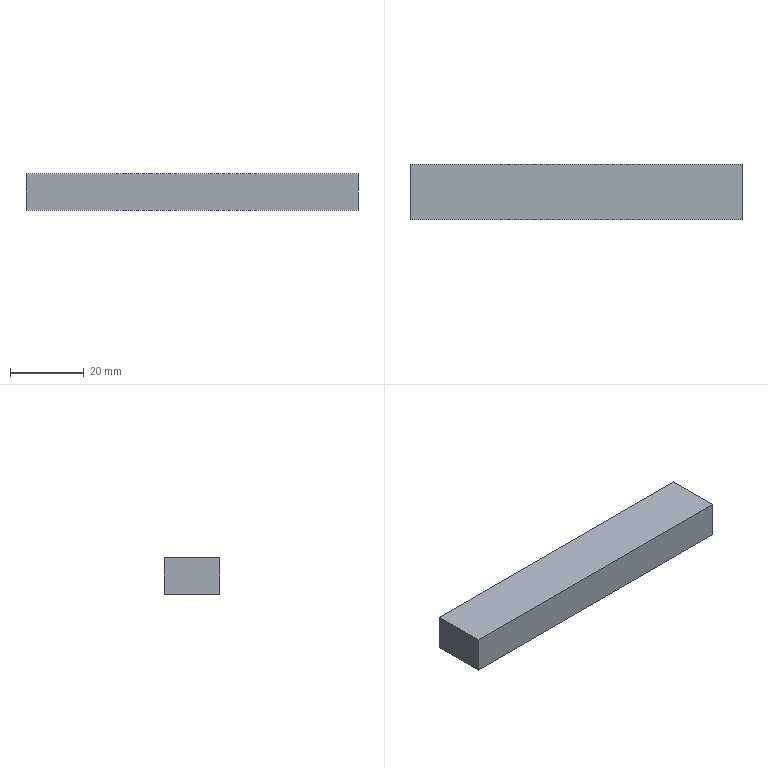Part | SolidWorks | features BaseBody 1 | 1 solid | 6 faces | box 90 x 15 x 10 mm | volume 13500 mm3 | plane 6
STEP:
#1=CARTESIAN_POINT('',(45.,-7.5,0.));
#2=VERTEX_POINT('',#1);
#3=CARTESIAN_POINT('',(45.,7.5,0.));
#4=VERTEX_POINT('',#3);
#5=CARTESIAN_POINT('',(45.,7.5,0.));
#6=DIRECTION('',(0.,1.,0.));
#7=VECTOR('',#6,1000.);
#8=LINE('',#5,#7);
#9=EDGE_CURVE('',#2,#4,#8,.T.);
#10=ORIENTED_EDGE('',*,*,#9,.T.);
#11=CARTESIAN_POINT('',(45.,7.5,10.));
#12=VERTEX_POINT('',#11);
#13=CARTESIAN_POINT('',(45.,7.5,10.));
#14=DIRECTION('',(0.,0.,-1.));
#15=VECTOR('',#14,1000.);
#16=LINE('',#13,#15);
#17=EDGE_CURVE('',#12,#4,#16,.T.);
#18=ORIENTED_EDGE('',*,*,#17,.F.);
#19=CARTESIAN_POINT('',(45.,-7.5,10.));
#20=VERTEX_POINT('',#19);
#21=CARTESIAN_POINT('',(45.,7.5,10.));
#22=DIRECTION('',(0.,1.,0.));
#23=VECTOR('',#22,1000.);
#24=LINE('',#21,#23);
#25=EDGE_CURVE('',#20,#12,#24,.T.);
#26=ORIENTED_EDGE('',*,*,#25,.F.);
#27=CARTESIAN_POINT('',(45.,-7.5,10.));
#28=DIRECTION('',(0.,0.,-1.));
#29=VECTOR('',#28,1000.);
#30=LINE('',#27,#29);
#31=EDGE_CURVE('',#20,#2,#30,.T.);
#32=ORIENTED_EDGE('',*,*,#31,.T.);
#33=EDGE_LOOP('',(#10,#18,#26,#32));
#34=FACE_OUTER_BOUND('',#33,.T.);
#35=CARTESIAN_POINT('',(45.,7.5,10.));
#36=DIRECTION('',(-1.,0.,0.));
#37=DIRECTION('',(0.,0.,1.));
#38=AXIS2_PLACEMENT_3D('',#35,#36,#37);
#39=PLANE('',#38);
#40=ADVANCED_FACE('',(#34),#39,.F.);
#41=CARTESIAN_POINT('',(-45.,7.5,0.));
#42=VERTEX_POINT('',#41);
#43=CARTESIAN_POINT('',(-45.,7.5,0.));
#44=DIRECTION('',(-1.,0.,0.));
#45=VECTOR('',#44,1000.);
#46=LINE('',#43,#45);
#47=EDGE_CURVE('',#4,#42,#46,.T.);
#48=ORIENTED_EDGE('',*,*,#47,.T.);
#49=CARTESIAN_POINT('',(-45.,7.5,10.));
#50=VERTEX_POINT('',#49);
#51=CARTESIAN_POINT('',(-45.,7.5,10.));
#52=DIRECTION('',(0.,0.,-1.));
#53=VECTOR('',#52,1000.);
#54=LINE('',#51,#53);
#55=EDGE_CURVE('',#50,#42,#54,.T.);
#56=ORIENTED_EDGE('',*,*,#55,.F.);
#57=CARTESIAN_POINT('',(-45.,7.5,10.));
#58=DIRECTION('',(-1.,0.,0.));
#59=VECTOR('',#58,1000.);
#60=LINE('',#57,#59);
#61=EDGE_CURVE('',#12,#50,#60,.T.);
#62=ORIENTED_EDGE('',*,*,#61,.F.);
#63=ORIENTED_EDGE('',*,*,#17,.T.);
#64=EDGE_LOOP('',(#48,#56,#62,#63));
#65=FACE_OUTER_BOUND('',#64,.T.);
#66=CARTESIAN_POINT('',(-45.,7.5,10.));
#67=DIRECTION('',(0.,-1.,0.));
#68=DIRECTION('',(0.,0.,-1.));
#69=AXIS2_PLACEMENT_3D('',#66,#67,#68);
#70=PLANE('',#69);
#71=ADVANCED_FACE('',(#65),#70,.F.);
#72=CARTESIAN_POINT('',(-45.,-7.5,0.));
#73=VERTEX_POINT('',#72);
#74=CARTESIAN_POINT('',(-45.,7.5,0.));
#75=DIRECTION('',(0.,-1.,0.));
#76=VECTOR('',#75,1000.);
#77=LINE('',#74,#76);
#78=EDGE_CURVE('',#42,#73,#77,.T.);
#79=ORIENTED_EDGE('',*,*,#78,.T.);
#80=CARTESIAN_POINT('',(-45.,-7.5,10.));
#81=VERTEX_POINT('',#80);
#82=CARTESIAN_POINT('',(-45.,-7.5,10.));
#83=DIRECTION('',(0.,0.,-1.));
#84=VECTOR('',#83,1000.);
#85=LINE('',#82,#84);
#86=EDGE_CURVE('',#81,#73,#85,.T.);
#87=ORIENTED_EDGE('',*,*,#86,.F.);
#88=CARTESIAN_POINT('',(-45.,7.5,10.));
#89=DIRECTION('',(0.,-1.,0.));
#90=VECTOR('',#89,1000.);
#91=LINE('',#88,#90);
#92=EDGE_CURVE('',#50,#81,#91,.T.);
#93=ORIENTED_EDGE('',*,*,#92,.F.);
#94=ORIENTED_EDGE('',*,*,#55,.T.);
#95=EDGE_LOOP('',(#79,#87,#93,#94));
#96=FACE_OUTER_BOUND('',#95,.T.);
#97=CARTESIAN_POINT('',(-45.,7.5,10.));
#98=DIRECTION('',(1.,0.,0.));
#99=DIRECTION('',(0.,0.,-1.));
#100=AXIS2_PLACEMENT_3D('',#97,#98,#99);
#101=PLANE('',#100);
#102=ADVANCED_FACE('',(#96),#101,.F.);
#103=CARTESIAN_POINT('',(-45.,-7.5,0.));
#104=DIRECTION('',(1.,0.,0.));
#105=VECTOR('',#104,1000.);
#106=LINE('',#103,#105);
#107=EDGE_CURVE('',#73,#2,#106,.T.);
#108=ORIENTED_EDGE('',*,*,#107,.T.);
#109=ORIENTED_EDGE('',*,*,#31,.F.);
#110=CARTESIAN_POINT('',(-45.,-7.5,10.));
#111=DIRECTION('',(1.,0.,0.));
#112=VECTOR('',#111,1000.);
#113=LINE('',#110,#112);
#114=EDGE_CURVE('',#81,#20,#113,.T.);
#115=ORIENTED_EDGE('',*,*,#114,.F.);
#116=ORIENTED_EDGE('',*,*,#86,.T.);
#117=EDGE_LOOP('',(#108,#109,#115,#116));
#118=FACE_OUTER_BOUND('',#117,.T.);
#119=CARTESIAN_POINT('',(-45.,-7.5,10.));
#120=DIRECTION('',(0.,1.,0.));
#121=DIRECTION('',(0.,0.,1.));
#122=AXIS2_PLACEMENT_3D('',#119,#120,#121);
#123=PLANE('',#122);
#124=ADVANCED_FACE('',(#118),#123,.F.);
#125=ORIENTED_EDGE('',*,*,#25,.T.);
#126=ORIENTED_EDGE('',*,*,#61,.T.);
#127=ORIENTED_EDGE('',*,*,#92,.T.);
#128=ORIENTED_EDGE('',*,*,#114,.T.);
#129=EDGE_LOOP('',(#125,#126,#127,#128));
#130=FACE_OUTER_BOUND('',#129,.T.);
#131=CARTESIAN_POINT('',(0.,0.,10.));
#132=DIRECTION('',(0.,0.,1.));
#133=DIRECTION('',(1.,0.,0.));
#134=AXIS2_PLACEMENT_3D('',#131,#132,#133);
#135=PLANE('',#134);
#136=ADVANCED_FACE('',(#130),#135,.T.);
#137=ORIENTED_EDGE('',*,*,#9,.F.);
#138=ORIENTED_EDGE('',*,*,#107,.F.);
#139=ORIENTED_EDGE('',*,*,#78,.F.);
#140=ORIENTED_EDGE('',*,*,#47,.F.);
#141=EDGE_LOOP('',(#137,#138,#139,#140));
#142=FACE_OUTER_BOUND('',#141,.T.);
#143=CARTESIAN_POINT('',(0.,0.,0.));
#144=DIRECTION('',(0.,0.,1.));
#145=DIRECTION('',(1.,0.,0.));
#146=AXIS2_PLACEMENT_3D('',#143,#144,#145);
#147=PLANE('',#146);
#148=ADVANCED_FACE('',(#142),#147,.F.);
#149=CLOSED_SHELL('',(#40,#71,#102,#124,#136,#148));
#150=MANIFOLD_SOLID_BREP('',#149);
#151=CARTESIAN_POINT('',(0.,0.,0.));
#152=DIRECTION('',(0.,0.,1.));
#153=DIRECTION('',(1.,0.,0.));
#154=AXIS2_PLACEMENT_3D('',#151,#152,#153);
#155=(LENGTH_UNIT()NAMED_UNIT(*)SI_UNIT(.MILLI.,.METRE.));
#156=UNCERTAINTY_MEASURE_WITH_UNIT(LENGTH_MEASURE(0.00001),#155,'','');
#157=(NAMED_UNIT(*)PLANE_ANGLE_UNIT()SI_UNIT($,.RADIAN.));
#158=(NAMED_UNIT(*)SI_UNIT($,.STERADIAN.)SOLID_ANGLE_UNIT());
#159=(GEOMETRIC_REPRESENTATION_CONTEXT(3)GLOBAL_UNCERTAINTY_ASSIGNED_CONTEXT((#156))GLOBAL_UNIT_ASSIGNED_CONTEXT((#155,#157,#158))REPRESENTATION_CONTEXT('',''));
#160=ADVANCED_BREP_SHAPE_REPRESENTATION('',(#150,#154),#159);